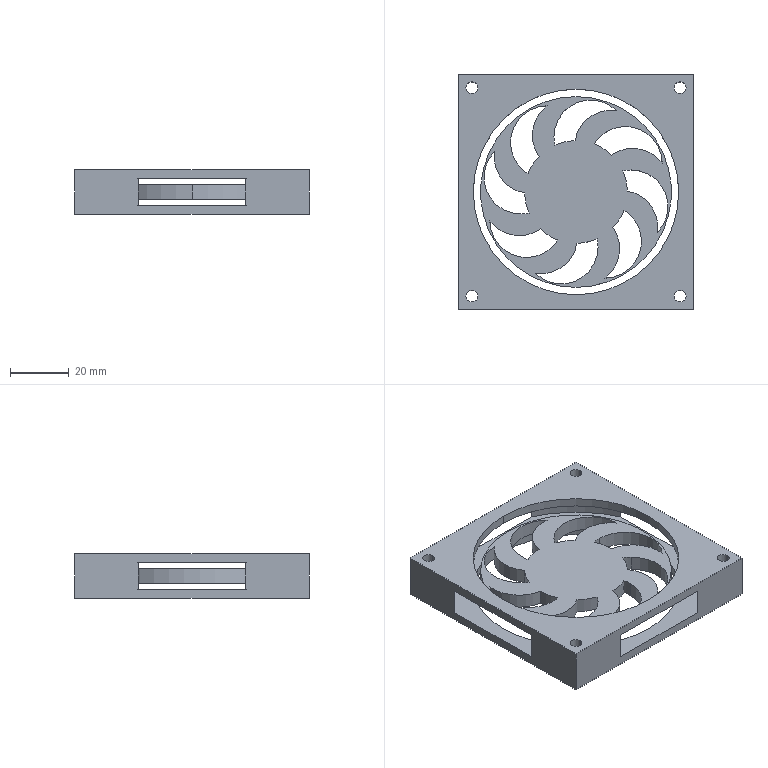Part | STEP file | 162-FENGSAN-220V-80X80.stp.STEP | 2 solids | 60 faces | box 80 x 80 x 15 mm | volume 31941 mm3 | cylinder 50 | plane 10 | commonest cylinder face diameters 25 x24 4 x8 35 x8 70 x4 88 x4 65 x2